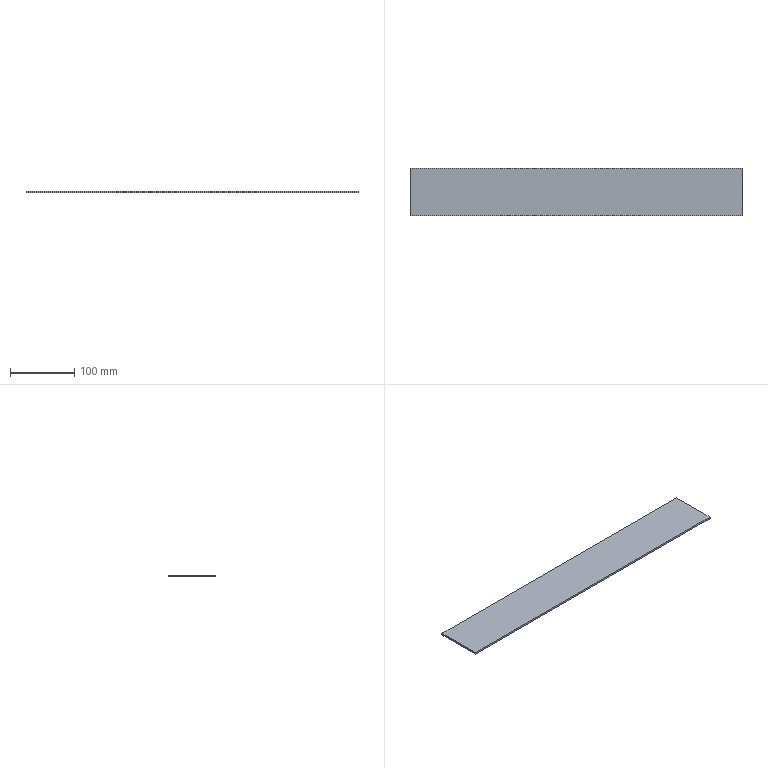Part | SolidWorks | features Extrusion 1 | 1 solid | 6 faces | box 515 x 73 x 3 mm | volume 112785 mm3 | plane 6
STEP:
#1=CARTESIAN_POINT('',(257.5,-36.5,0.));
#2=VERTEX_POINT('',#1);
#3=CARTESIAN_POINT('',(257.5,36.5,0.));
#4=VERTEX_POINT('',#3);
#5=CARTESIAN_POINT('',(257.5,36.5,0.));
#6=DIRECTION('',(0.,1.,0.));
#7=VECTOR('',#6,1000.);
#8=LINE('',#5,#7);
#9=EDGE_CURVE('',#2,#4,#8,.T.);
#10=ORIENTED_EDGE('',*,*,#9,.T.);
#11=CARTESIAN_POINT('',(257.5,36.5,3.));
#12=VERTEX_POINT('',#11);
#13=CARTESIAN_POINT('',(257.5,36.5,3.));
#14=DIRECTION('',(0.,0.,-1.));
#15=VECTOR('',#14,1000.);
#16=LINE('',#13,#15);
#17=EDGE_CURVE('',#12,#4,#16,.T.);
#18=ORIENTED_EDGE('',*,*,#17,.F.);
#19=CARTESIAN_POINT('',(257.5,-36.5,3.));
#20=VERTEX_POINT('',#19);
#21=CARTESIAN_POINT('',(257.5,36.5,3.));
#22=DIRECTION('',(0.,1.,0.));
#23=VECTOR('',#22,1000.);
#24=LINE('',#21,#23);
#25=EDGE_CURVE('',#20,#12,#24,.T.);
#26=ORIENTED_EDGE('',*,*,#25,.F.);
#27=CARTESIAN_POINT('',(257.5,-36.5,3.));
#28=DIRECTION('',(0.,0.,-1.));
#29=VECTOR('',#28,1000.);
#30=LINE('',#27,#29);
#31=EDGE_CURVE('',#20,#2,#30,.T.);
#32=ORIENTED_EDGE('',*,*,#31,.T.);
#33=EDGE_LOOP('',(#10,#18,#26,#32));
#34=FACE_OUTER_BOUND('',#33,.T.);
#35=CARTESIAN_POINT('',(257.5,36.5,3.));
#36=DIRECTION('',(-1.,0.,0.));
#37=DIRECTION('',(0.,0.,1.));
#38=AXIS2_PLACEMENT_3D('',#35,#36,#37);
#39=PLANE('',#38);
#40=ADVANCED_FACE('',(#34),#39,.F.);
#41=CARTESIAN_POINT('',(-257.5,36.5,0.));
#42=VERTEX_POINT('',#41);
#43=CARTESIAN_POINT('',(-257.5,36.5,0.));
#44=DIRECTION('',(-1.,0.,0.));
#45=VECTOR('',#44,1000.);
#46=LINE('',#43,#45);
#47=EDGE_CURVE('',#4,#42,#46,.T.);
#48=ORIENTED_EDGE('',*,*,#47,.T.);
#49=CARTESIAN_POINT('',(-257.5,36.5,3.));
#50=VERTEX_POINT('',#49);
#51=CARTESIAN_POINT('',(-257.5,36.5,3.));
#52=DIRECTION('',(0.,0.,-1.));
#53=VECTOR('',#52,1000.);
#54=LINE('',#51,#53);
#55=EDGE_CURVE('',#50,#42,#54,.T.);
#56=ORIENTED_EDGE('',*,*,#55,.F.);
#57=CARTESIAN_POINT('',(-257.5,36.5,3.));
#58=DIRECTION('',(-1.,0.,0.));
#59=VECTOR('',#58,1000.);
#60=LINE('',#57,#59);
#61=EDGE_CURVE('',#12,#50,#60,.T.);
#62=ORIENTED_EDGE('',*,*,#61,.F.);
#63=ORIENTED_EDGE('',*,*,#17,.T.);
#64=EDGE_LOOP('',(#48,#56,#62,#63));
#65=FACE_OUTER_BOUND('',#64,.T.);
#66=CARTESIAN_POINT('',(-257.5,36.5,3.));
#67=DIRECTION('',(0.,-1.,0.));
#68=DIRECTION('',(0.,0.,-1.));
#69=AXIS2_PLACEMENT_3D('',#66,#67,#68);
#70=PLANE('',#69);
#71=ADVANCED_FACE('',(#65),#70,.F.);
#72=CARTESIAN_POINT('',(-257.5,-36.5,0.));
#73=VERTEX_POINT('',#72);
#74=CARTESIAN_POINT('',(-257.5,36.5,0.));
#75=DIRECTION('',(0.,-1.,0.));
#76=VECTOR('',#75,1000.);
#77=LINE('',#74,#76);
#78=EDGE_CURVE('',#42,#73,#77,.T.);
#79=ORIENTED_EDGE('',*,*,#78,.T.);
#80=CARTESIAN_POINT('',(-257.5,-36.5,3.));
#81=VERTEX_POINT('',#80);
#82=CARTESIAN_POINT('',(-257.5,-36.5,3.));
#83=DIRECTION('',(0.,0.,-1.));
#84=VECTOR('',#83,1000.);
#85=LINE('',#82,#84);
#86=EDGE_CURVE('',#81,#73,#85,.T.);
#87=ORIENTED_EDGE('',*,*,#86,.F.);
#88=CARTESIAN_POINT('',(-257.5,36.5,3.));
#89=DIRECTION('',(0.,-1.,0.));
#90=VECTOR('',#89,1000.);
#91=LINE('',#88,#90);
#92=EDGE_CURVE('',#50,#81,#91,.T.);
#93=ORIENTED_EDGE('',*,*,#92,.F.);
#94=ORIENTED_EDGE('',*,*,#55,.T.);
#95=EDGE_LOOP('',(#79,#87,#93,#94));
#96=FACE_OUTER_BOUND('',#95,.T.);
#97=CARTESIAN_POINT('',(-257.5,36.5,3.));
#98=DIRECTION('',(1.,0.,0.));
#99=DIRECTION('',(0.,0.,-1.));
#100=AXIS2_PLACEMENT_3D('',#97,#98,#99);
#101=PLANE('',#100);
#102=ADVANCED_FACE('',(#96),#101,.F.);
#103=CARTESIAN_POINT('',(-257.5,-36.5,0.));
#104=DIRECTION('',(1.,0.,0.));
#105=VECTOR('',#104,1000.);
#106=LINE('',#103,#105);
#107=EDGE_CURVE('',#73,#2,#106,.T.);
#108=ORIENTED_EDGE('',*,*,#107,.T.);
#109=ORIENTED_EDGE('',*,*,#31,.F.);
#110=CARTESIAN_POINT('',(-257.5,-36.5,3.));
#111=DIRECTION('',(1.,0.,0.));
#112=VECTOR('',#111,1000.);
#113=LINE('',#110,#112);
#114=EDGE_CURVE('',#81,#20,#113,.T.);
#115=ORIENTED_EDGE('',*,*,#114,.F.);
#116=ORIENTED_EDGE('',*,*,#86,.T.);
#117=EDGE_LOOP('',(#108,#109,#115,#116));
#118=FACE_OUTER_BOUND('',#117,.T.);
#119=CARTESIAN_POINT('',(-257.5,-36.5,3.));
#120=DIRECTION('',(0.,1.,0.));
#121=DIRECTION('',(0.,0.,1.));
#122=AXIS2_PLACEMENT_3D('',#119,#120,#121);
#123=PLANE('',#122);
#124=ADVANCED_FACE('',(#118),#123,.F.);
#125=ORIENTED_EDGE('',*,*,#25,.T.);
#126=ORIENTED_EDGE('',*,*,#61,.T.);
#127=ORIENTED_EDGE('',*,*,#92,.T.);
#128=ORIENTED_EDGE('',*,*,#114,.T.);
#129=EDGE_LOOP('',(#125,#126,#127,#128));
#130=FACE_OUTER_BOUND('',#129,.T.);
#131=CARTESIAN_POINT('',(0.,0.,3.));
#132=DIRECTION('',(0.,0.,1.));
#133=DIRECTION('',(1.,0.,0.));
#134=AXIS2_PLACEMENT_3D('',#131,#132,#133);
#135=PLANE('',#134);
#136=ADVANCED_FACE('',(#130),#135,.T.);
#137=ORIENTED_EDGE('',*,*,#9,.F.);
#138=ORIENTED_EDGE('',*,*,#107,.F.);
#139=ORIENTED_EDGE('',*,*,#78,.F.);
#140=ORIENTED_EDGE('',*,*,#47,.F.);
#141=EDGE_LOOP('',(#137,#138,#139,#140));
#142=FACE_OUTER_BOUND('',#141,.T.);
#143=CARTESIAN_POINT('',(0.,0.,0.));
#144=DIRECTION('',(0.,0.,1.));
#145=DIRECTION('',(1.,0.,0.));
#146=AXIS2_PLACEMENT_3D('',#143,#144,#145);
#147=PLANE('',#146);
#148=ADVANCED_FACE('',(#142),#147,.F.);
#149=CLOSED_SHELL('',(#40,#71,#102,#124,#136,#148));
#150=MANIFOLD_SOLID_BREP('',#149);
#151=CARTESIAN_POINT('',(0.,0.,0.));
#152=DIRECTION('',(0.,0.,1.));
#153=DIRECTION('',(1.,0.,0.));
#154=AXIS2_PLACEMENT_3D('',#151,#152,#153);
#155=(LENGTH_UNIT()NAMED_UNIT(*)SI_UNIT(.MILLI.,.METRE.));
#156=UNCERTAINTY_MEASURE_WITH_UNIT(LENGTH_MEASURE(0.00001),#155,'','');
#157=(NAMED_UNIT(*)PLANE_ANGLE_UNIT()SI_UNIT($,.RADIAN.));
#158=(NAMED_UNIT(*)SI_UNIT($,.STERADIAN.)SOLID_ANGLE_UNIT());
#159=(GEOMETRIC_REPRESENTATION_CONTEXT(3)GLOBAL_UNCERTAINTY_ASSIGNED_CONTEXT((#156))GLOBAL_UNIT_ASSIGNED_CONTEXT((#155,#157,#158))REPRESENTATION_CONTEXT('',''));
#160=ADVANCED_BREP_SHAPE_REPRESENTATION('',(#150,#154),#159);